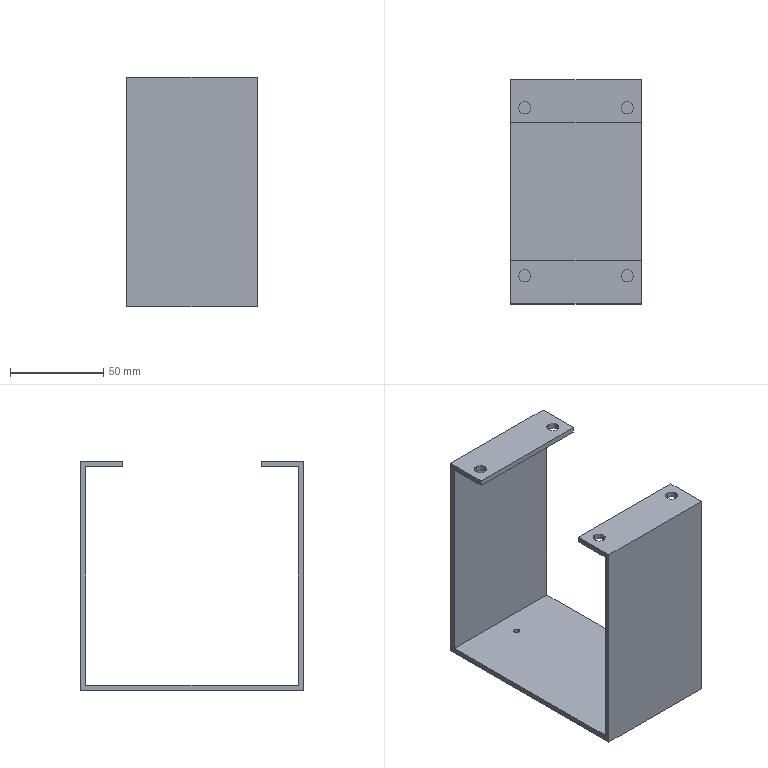Part | SolidWorks | features 3DProfileFeature 1, BaseBody 1, HoleWzd 1 | 1 solid | 26 faces | box 70 x 120 x 123 mm | volume 83550 mm3 | plane 14 | cylinder 12 | commonest cylinder face diameters 6.5 x8 3.3 x4
STEP:
#1=CARTESIAN_POINT('',(-36.65,15.,3.));
#2=VERTEX_POINT('',#1);
#3=CARTESIAN_POINT('',(-33.35,15.,3.));
#4=VERTEX_POINT('',#3);
#5=CARTESIAN_POINT('',(-35.,15.,3.));
#6=DIRECTION('',(0.,0.,1.));
#7=DIRECTION('',(1.,0.,0.));
#8=AXIS2_PLACEMENT_3D('',#5,#6,#7);
#9=CIRCLE('',#8,1.65);
#10=EDGE_CURVE('',#2,#4,#9,.T.);
#11=ORIENTED_EDGE('',*,*,#10,.T.);
#12=CARTESIAN_POINT('',(-33.35,15.,0.));
#13=VERTEX_POINT('',#12);
#14=CARTESIAN_POINT('',(-33.35,15.,0.));
#15=DIRECTION('',(0.,0.,-1.));
#16=VECTOR('',#15,1000.);
#17=LINE('',#14,#16);
#18=EDGE_CURVE('',#4,#13,#17,.T.);
#19=ORIENTED_EDGE('',*,*,#18,.T.);
#20=CARTESIAN_POINT('',(-36.65,15.,0.));
#21=VERTEX_POINT('',#20);
#22=CARTESIAN_POINT('',(-35.,15.,0.));
#23=DIRECTION('',(0.,0.,-1.));
#24=DIRECTION('',(-1.,0.,0.));
#25=AXIS2_PLACEMENT_3D('',#22,#23,#24);
#26=CIRCLE('',#25,1.65);
#27=EDGE_CURVE('',#13,#21,#26,.T.);
#28=ORIENTED_EDGE('',*,*,#27,.T.);
#29=CARTESIAN_POINT('',(-36.65,15.,0.));
#30=DIRECTION('',(0.,0.,-1.));
#31=VECTOR('',#30,1000.);
#32=LINE('',#29,#31);
#33=EDGE_CURVE('',#2,#21,#32,.T.);
#34=ORIENTED_EDGE('',*,*,#33,.F.);
#35=EDGE_LOOP('',(#11,#19,#28,#34));
#36=FACE_OUTER_BOUND('',#35,.T.);
#37=CARTESIAN_POINT('',(-35.,15.,0.));
#38=DIRECTION('',(0.,0.,-1.));
#39=DIRECTION('',(-1.,0.,0.));
#40=AXIS2_PLACEMENT_3D('',#37,#38,#39);
#41=CYLINDRICAL_SURFACE('',#40,1.65);
#42=ADVANCED_FACE('',(#36),#41,.F.);
#43=CARTESIAN_POINT('',(-36.65,105.,3.));
#44=VERTEX_POINT('',#43);
#45=CARTESIAN_POINT('',(-33.35,105.,3.));
#46=VERTEX_POINT('',#45);
#47=CARTESIAN_POINT('',(-35.,105.,3.));
#48=DIRECTION('',(0.,0.,1.));
#49=DIRECTION('',(1.,0.,0.));
#50=AXIS2_PLACEMENT_3D('',#47,#48,#49);
#51=CIRCLE('',#50,1.65);
#52=EDGE_CURVE('',#44,#46,#51,.T.);
#53=ORIENTED_EDGE('',*,*,#52,.T.);
#54=CARTESIAN_POINT('',(-33.35,105.,0.));
#55=VERTEX_POINT('',#54);
#56=CARTESIAN_POINT('',(-33.35,105.,0.));
#57=DIRECTION('',(0.,0.,-1.));
#58=VECTOR('',#57,1000.);
#59=LINE('',#56,#58);
#60=EDGE_CURVE('',#46,#55,#59,.T.);
#61=ORIENTED_EDGE('',*,*,#60,.T.);
#62=CARTESIAN_POINT('',(-36.65,105.,0.));
#63=VERTEX_POINT('',#62);
#64=CARTESIAN_POINT('',(-35.,105.,0.));
#65=DIRECTION('',(0.,0.,-1.));
#66=DIRECTION('',(-1.,0.,0.));
#67=AXIS2_PLACEMENT_3D('',#64,#65,#66);
#68=CIRCLE('',#67,1.65);
#69=EDGE_CURVE('',#55,#63,#68,.T.);
#70=ORIENTED_EDGE('',*,*,#69,.T.);
#71=CARTESIAN_POINT('',(-36.65,105.,0.));
#72=DIRECTION('',(0.,0.,-1.));
#73=VECTOR('',#72,1000.);
#74=LINE('',#71,#73);
#75=EDGE_CURVE('',#44,#63,#74,.T.);
#76=ORIENTED_EDGE('',*,*,#75,.F.);
#77=EDGE_LOOP('',(#53,#61,#70,#76));
#78=FACE_OUTER_BOUND('',#77,.T.);
#79=CARTESIAN_POINT('',(-35.,105.,0.));
#80=DIRECTION('',(0.,0.,-1.));
#81=DIRECTION('',(-1.,0.,0.));
#82=AXIS2_PLACEMENT_3D('',#79,#80,#81);
#83=CYLINDRICAL_SURFACE('',#82,1.65);
#84=ADVANCED_FACE('',(#78),#83,.F.);
#85=CARTESIAN_POINT('',(-7.5,101.75,120.));
#86=VERTEX_POINT('',#85);
#87=CARTESIAN_POINT('',(-7.5,108.25,120.));
#88=VERTEX_POINT('',#87);
#89=CARTESIAN_POINT('',(-7.5,105.,120.));
#90=DIRECTION('',(0.,0.,-1.));
#91=DIRECTION('',(0.,-1.,0.));
#92=AXIS2_PLACEMENT_3D('',#89,#90,#91);
#93=CIRCLE('',#92,3.25);
#94=EDGE_CURVE('',#86,#88,#93,.T.);
#95=ORIENTED_EDGE('',*,*,#94,.T.);
#96=CARTESIAN_POINT('',(-7.5,108.25,123.));
#97=VERTEX_POINT('',#96);
#98=CARTESIAN_POINT('',(-7.5,108.25,120.));
#99=DIRECTION('',(0.,0.,1.));
#100=VECTOR('',#99,1000.);
#101=LINE('',#98,#100);
#102=EDGE_CURVE('',#88,#97,#101,.T.);
#103=ORIENTED_EDGE('',*,*,#102,.T.);
#104=CARTESIAN_POINT('',(-7.5,101.75,123.));
#105=VERTEX_POINT('',#104);
#106=CARTESIAN_POINT('',(-7.5,105.,123.));
#107=DIRECTION('',(0.,0.,1.));
#108=DIRECTION('',(0.,-1.,0.));
#109=AXIS2_PLACEMENT_3D('',#106,#107,#108);
#110=CIRCLE('',#109,3.25);
#111=EDGE_CURVE('',#97,#105,#110,.T.);
#112=ORIENTED_EDGE('',*,*,#111,.T.);
#113=CARTESIAN_POINT('',(-7.5,101.75,120.));
#114=DIRECTION('',(0.,0.,1.));
#115=VECTOR('',#114,1000.);
#116=LINE('',#113,#115);
#117=EDGE_CURVE('',#86,#105,#116,.T.);
#118=ORIENTED_EDGE('',*,*,#117,.F.);
#119=EDGE_LOOP('',(#95,#103,#112,#118));
#120=FACE_OUTER_BOUND('',#119,.T.);
#121=CARTESIAN_POINT('',(-7.5,105.,120.));
#122=DIRECTION('',(0.,0.,1.));
#123=DIRECTION('',(0.,-1.,0.));
#124=AXIS2_PLACEMENT_3D('',#121,#122,#123);
#125=CYLINDRICAL_SURFACE('',#124,3.25);
#126=ADVANCED_FACE('',(#120),#125,.F.);
#127=CARTESIAN_POINT('',(-62.5,101.75,120.));
#128=VERTEX_POINT('',#127);
#129=CARTESIAN_POINT('',(-62.5,108.25,120.));
#130=VERTEX_POINT('',#129);
#131=CARTESIAN_POINT('',(-62.5,105.,120.));
#132=DIRECTION('',(0.,0.,-1.));
#133=DIRECTION('',(0.,-1.,0.));
#134=AXIS2_PLACEMENT_3D('',#131,#132,#133);
#135=CIRCLE('',#134,3.25);
#136=EDGE_CURVE('',#128,#130,#135,.T.);
#137=ORIENTED_EDGE('',*,*,#136,.T.);
#138=CARTESIAN_POINT('',(-62.5,108.25,123.));
#139=VERTEX_POINT('',#138);
#140=CARTESIAN_POINT('',(-62.5,108.25,120.));
#141=DIRECTION('',(0.,0.,1.));
#142=VECTOR('',#141,1000.);
#143=LINE('',#140,#142);
#144=EDGE_CURVE('',#130,#139,#143,.T.);
#145=ORIENTED_EDGE('',*,*,#144,.T.);
#146=CARTESIAN_POINT('',(-62.5,101.75,123.));
#147=VERTEX_POINT('',#146);
#148=CARTESIAN_POINT('',(-62.5,105.,123.));
#149=DIRECTION('',(0.,0.,-1.));
#150=DIRECTION('',(0.,-1.,0.));
#151=AXIS2_PLACEMENT_3D('',#148,#149,#150);
#152=CIRCLE('',#151,3.25);
#153=EDGE_CURVE('',#147,#139,#152,.T.);
#154=ORIENTED_EDGE('',*,*,#153,.F.);
#155=CARTESIAN_POINT('',(-62.5,101.75,120.));
#156=DIRECTION('',(0.,0.,1.));
#157=VECTOR('',#156,1000.);
#158=LINE('',#155,#157);
#159=EDGE_CURVE('',#128,#147,#158,.T.);
#160=ORIENTED_EDGE('',*,*,#159,.F.);
#161=EDGE_LOOP('',(#137,#145,#154,#160));
#162=FACE_OUTER_BOUND('',#161,.T.);
#163=CARTESIAN_POINT('',(-62.5,105.,120.));
#164=DIRECTION('',(0.,0.,1.));
#165=DIRECTION('',(0.,-1.,0.));
#166=AXIS2_PLACEMENT_3D('',#163,#164,#165);
#167=CYLINDRICAL_SURFACE('',#166,3.25);
#168=ADVANCED_FACE('',(#162),#167,.F.);
#169=CARTESIAN_POINT('',(-7.5,11.75,120.));
#170=VERTEX_POINT('',#169);
#171=CARTESIAN_POINT('',(-7.5,18.25,120.));
#172=VERTEX_POINT('',#171);
#173=CARTESIAN_POINT('',(-7.5,15.,120.));
#174=DIRECTION('',(0.,0.,-1.));
#175=DIRECTION('',(0.,-1.,0.));
#176=AXIS2_PLACEMENT_3D('',#173,#174,#175);
#177=CIRCLE('',#176,3.25);
#178=EDGE_CURVE('',#170,#172,#177,.T.);
#179=ORIENTED_EDGE('',*,*,#178,.T.);
#180=CARTESIAN_POINT('',(-7.5,18.25,123.));
#181=VERTEX_POINT('',#180);
#182=CARTESIAN_POINT('',(-7.5,18.25,120.));
#183=DIRECTION('',(0.,0.,1.));
#184=VECTOR('',#183,1000.);
#185=LINE('',#182,#184);
#186=EDGE_CURVE('',#172,#181,#185,.T.);
#187=ORIENTED_EDGE('',*,*,#186,.T.);
#188=CARTESIAN_POINT('',(-7.5,11.75,123.));
#189=VERTEX_POINT('',#188);
#190=CARTESIAN_POINT('',(-7.5,15.,123.));
#191=DIRECTION('',(0.,0.,-1.));
#192=DIRECTION('',(0.,-1.,0.));
#193=AXIS2_PLACEMENT_3D('',#190,#191,#192);
#194=CIRCLE('',#193,3.25);
#195=EDGE_CURVE('',#189,#181,#194,.T.);
#196=ORIENTED_EDGE('',*,*,#195,.F.);
#197=CARTESIAN_POINT('',(-7.5,11.75,120.));
#198=DIRECTION('',(0.,0.,1.));
#199=VECTOR('',#198,1000.);
#200=LINE('',#197,#199);
#201=EDGE_CURVE('',#170,#189,#200,.T.);
#202=ORIENTED_EDGE('',*,*,#201,.F.);
#203=EDGE_LOOP('',(#179,#187,#196,#202));
#204=FACE_OUTER_BOUND('',#203,.T.);
#205=CARTESIAN_POINT('',(-7.5,15.,120.));
#206=DIRECTION('',(0.,0.,1.));
#207=DIRECTION('',(0.,-1.,0.));
#208=AXIS2_PLACEMENT_3D('',#205,#206,#207);
#209=CYLINDRICAL_SURFACE('',#208,3.25);
#210=ADVANCED_FACE('',(#204),#209,.F.);
#211=CARTESIAN_POINT('',(-62.5,11.75,120.));
#212=VERTEX_POINT('',#211);
#213=CARTESIAN_POINT('',(-62.5,18.25,120.));
#214=VERTEX_POINT('',#213);
#215=CARTESIAN_POINT('',(-62.5,15.,120.));
#216=DIRECTION('',(0.,0.,-1.));
#217=DIRECTION('',(0.,-1.,0.));
#218=AXIS2_PLACEMENT_3D('',#215,#216,#217);
#219=CIRCLE('',#218,3.25);
#220=EDGE_CURVE('',#212,#214,#219,.T.);
#221=ORIENTED_EDGE('',*,*,#220,.T.);
#222=CARTESIAN_POINT('',(-62.5,18.25,123.));
#223=VERTEX_POINT('',#222);
#224=CARTESIAN_POINT('',(-62.5,18.25,120.));
#225=DIRECTION('',(0.,0.,1.));
#226=VECTOR('',#225,1000.);
#227=LINE('',#224,#226);
#228=EDGE_CURVE('',#214,#223,#227,.T.);
#229=ORIENTED_EDGE('',*,*,#228,.T.);
#230=CARTESIAN_POINT('',(-62.5,11.75,123.));
#231=VERTEX_POINT('',#230);
#232=CARTESIAN_POINT('',(-62.5,15.,123.));
#233=DIRECTION('',(0.,0.,-1.));
#234=DIRECTION('',(0.,-1.,0.));
#235=AXIS2_PLACEMENT_3D('',#232,#233,#234);
#236=CIRCLE('',#235,3.25);
#237=EDGE_CURVE('',#231,#223,#236,.T.);
#238=ORIENTED_EDGE('',*,*,#237,.F.);
#239=CARTESIAN_POINT('',(-62.5,11.75,120.));
#240=DIRECTION('',(0.,0.,1.));
#241=VECTOR('',#240,1000.);
#242=LINE('',#239,#241);
#243=EDGE_CURVE('',#212,#231,#242,.T.);
#244=ORIENTED_EDGE('',*,*,#243,.F.);
#245=EDGE_LOOP('',(#221,#229,#238,#244));
#246=FACE_OUTER_BOUND('',#245,.T.);
#247=CARTESIAN_POINT('',(-62.5,15.,120.));
#248=DIRECTION('',(0.,0.,1.));
#249=DIRECTION('',(0.,-1.,0.));
#250=AXIS2_PLACEMENT_3D('',#247,#248,#249);
#251=CYLINDRICAL_SURFACE('',#250,3.25);
#252=ADVANCED_FACE('',(#246),#251,.F.);
#253=ORIENTED_EDGE('',*,*,#102,.F.);
#254=CARTESIAN_POINT('',(-7.5,105.,120.));
#255=DIRECTION('',(0.,0.,-1.));
#256=DIRECTION('',(0.,-1.,0.));
#257=AXIS2_PLACEMENT_3D('',#254,#255,#256);
#258=CIRCLE('',#257,3.25);
#259=EDGE_CURVE('',#88,#86,#258,.T.);
#260=ORIENTED_EDGE('',*,*,#259,.T.);
#261=ORIENTED_EDGE('',*,*,#117,.T.);
#262=CARTESIAN_POINT('',(-7.5,105.,123.));
#263=DIRECTION('',(0.,0.,1.));
#264=DIRECTION('',(0.,-1.,0.));
#265=AXIS2_PLACEMENT_3D('',#262,#263,#264);
#266=CIRCLE('',#265,3.25);
#267=EDGE_CURVE('',#105,#97,#266,.T.);
#268=ORIENTED_EDGE('',*,*,#267,.T.);
#269=EDGE_LOOP('',(#253,#260,#261,#268));
#270=FACE_OUTER_BOUND('',#269,.T.);
#271=CARTESIAN_POINT('',(-7.5,105.,120.));
#272=DIRECTION('',(0.,0.,1.));
#273=DIRECTION('',(0.,-1.,0.));
#274=AXIS2_PLACEMENT_3D('',#271,#272,#273);
#275=CYLINDRICAL_SURFACE('',#274,3.25);
#276=ADVANCED_FACE('',(#270),#275,.F.);
#277=ORIENTED_EDGE('',*,*,#153,.T.);
#278=CARTESIAN_POINT('',(-62.5,105.,123.));
#279=DIRECTION('',(0.,0.,-1.));
#280=DIRECTION('',(0.,-1.,0.));
#281=AXIS2_PLACEMENT_3D('',#278,#279,#280);
#282=CIRCLE('',#281,3.25);
#283=EDGE_CURVE('',#139,#147,#282,.T.);
#284=ORIENTED_EDGE('',*,*,#283,.T.);
#285=EDGE_LOOP('',(#277,#284));
#286=FACE_BOUND('',#285,.T.);
#287=ORIENTED_EDGE('',*,*,#267,.F.);
#288=ORIENTED_EDGE('',*,*,#111,.F.);
#289=EDGE_LOOP('',(#287,#288));
#290=FACE_BOUND('',#289,.T.);
#291=CARTESIAN_POINT('',(0.,97.,123.));
#292=VERTEX_POINT('',#291);
#293=CARTESIAN_POINT('',(0.,120.,123.));
#294=VERTEX_POINT('',#293);
#295=CARTESIAN_POINT('',(0.,108.5,123.));
#296=DIRECTION('',(0.,1.,0.));
#297=VECTOR('',#296,1000.);
#298=LINE('',#295,#297);
#299=EDGE_CURVE('',#292,#294,#298,.T.);
#300=ORIENTED_EDGE('',*,*,#299,.T.);
#301=CARTESIAN_POINT('',(-70.,120.,123.));
#302=VERTEX_POINT('',#301);
#303=CARTESIAN_POINT('',(-35.,120.,123.));
#304=DIRECTION('',(-1.,0.,0.));
#305=VECTOR('',#304,1000.);
#306=LINE('',#303,#305);
#307=EDGE_CURVE('',#294,#302,#306,.T.);
#308=ORIENTED_EDGE('',*,*,#307,.T.);
#309=CARTESIAN_POINT('',(-70.,97.,123.));
#310=VERTEX_POINT('',#309);
#311=CARTESIAN_POINT('',(-70.,108.5,123.));
#312=DIRECTION('',(0.,-1.,0.));
#313=VECTOR('',#312,1000.);
#314=LINE('',#311,#313);
#315=EDGE_CURVE('',#302,#310,#314,.T.);
#316=ORIENTED_EDGE('',*,*,#315,.T.);
#317=CARTESIAN_POINT('',(-35.,97.,123.));
#318=DIRECTION('',(1.,0.,0.));
#319=VECTOR('',#318,1000.);
#320=LINE('',#317,#319);
#321=EDGE_CURVE('',#310,#292,#320,.T.);
#322=ORIENTED_EDGE('',*,*,#321,.T.);
#323=EDGE_LOOP('',(#300,#308,#316,#322));
#324=FACE_OUTER_BOUND('',#323,.T.);
#325=CARTESIAN_POINT('',(-70.,97.,123.));
#326=DIRECTION('',(0.,0.,1.));
#327=DIRECTION('',(1.,0.,0.));
#328=AXIS2_PLACEMENT_3D('',#325,#326,#327);
#329=PLANE('',#328);
#330=ADVANCED_FACE('',(#286,#290,#324),#329,.T.);
#331=ORIENTED_EDGE('',*,*,#136,.F.);
#332=CARTESIAN_POINT('',(-62.5,105.,120.));
#333=DIRECTION('',(0.,0.,-1.));
#334=DIRECTION('',(0.,-1.,0.));
#335=AXIS2_PLACEMENT_3D('',#332,#333,#334);
#336=CIRCLE('',#335,3.25);
#337=EDGE_CURVE('',#130,#128,#336,.T.);
#338=ORIENTED_EDGE('',*,*,#337,.F.);
#339=EDGE_LOOP('',(#331,#338));
#340=FACE_BOUND('',#339,.T.);
#341=ORIENTED_EDGE('',*,*,#94,.F.);
#342=ORIENTED_EDGE('',*,*,#259,.F.);
#343=EDGE_LOOP('',(#341,#342));
#344=FACE_BOUND('',#343,.T.);
#345=CARTESIAN_POINT('',(0.,117.,120.));
#346=VERTEX_POINT('',#345);
#347=CARTESIAN_POINT('',(-70.,117.,120.));
#348=VERTEX_POINT('',#347);
#349=CARTESIAN_POINT('',(-35.,117.,120.));
#350=DIRECTION('',(-1.,0.,0.));
#351=VECTOR('',#350,1000.);
#352=LINE('',#349,#351);
#353=EDGE_CURVE('',#346,#348,#352,.T.);
#354=ORIENTED_EDGE('',*,*,#353,.F.);
#355=CARTESIAN_POINT('',(0.,97.,120.));
#356=VERTEX_POINT('',#355);
#357=CARTESIAN_POINT('',(0.,107.,120.));
#358=DIRECTION('',(0.,1.,0.));
#359=VECTOR('',#358,1000.);
#360=LINE('',#357,#359);
#361=EDGE_CURVE('',#356,#346,#360,.T.);
#362=ORIENTED_EDGE('',*,*,#361,.F.);
#363=CARTESIAN_POINT('',(-70.,97.,120.));
#364=VERTEX_POINT('',#363);
#365=CARTESIAN_POINT('',(-35.,97.,120.));
#366=DIRECTION('',(1.,0.,0.));
#367=VECTOR('',#366,1000.);
#368=LINE('',#365,#367);
#369=EDGE_CURVE('',#364,#356,#368,.T.);
#370=ORIENTED_EDGE('',*,*,#369,.F.);
#371=CARTESIAN_POINT('',(-70.,107.,120.));
#372=DIRECTION('',(0.,-1.,0.));
#373=VECTOR('',#372,1000.);
#374=LINE('',#371,#373);
#375=EDGE_CURVE('',#348,#364,#374,.T.);
#376=ORIENTED_EDGE('',*,*,#375,.F.);
#377=EDGE_LOOP('',(#354,#362,#370,#376));
#378=FACE_OUTER_BOUND('',#377,.T.);
#379=CARTESIAN_POINT('',(-70.,97.,120.));
#380=DIRECTION('',(0.,0.,1.));
#381=DIRECTION('',(1.,0.,0.));
#382=AXIS2_PLACEMENT_3D('',#379,#380,#381);
#383=PLANE('',#382);
#384=ADVANCED_FACE('',(#340,#344,#378),#383,.F.);
#385=ORIENTED_EDGE('',*,*,#144,.F.);
#386=ORIENTED_EDGE('',*,*,#337,.T.);
#387=ORIENTED_EDGE('',*,*,#159,.T.);
#388=ORIENTED_EDGE('',*,*,#283,.F.);
#389=EDGE_LOOP('',(#385,#386,#387,#388));
#390=FACE_OUTER_BOUND('',#389,.T.);
#391=CARTESIAN_POINT('',(-62.5,105.,120.));
#392=DIRECTION('',(0.,0.,1.));
#393=DIRECTION('',(0.,-1.,0.));
#394=AXIS2_PLACEMENT_3D('',#391,#392,#393);
#395=CYLINDRICAL_SURFACE('',#394,3.25);
#396=ADVANCED_FACE('',(#390),#395,.F.);
#397=CARTESIAN_POINT('',(-70.,120.,0.));
#398=VERTEX_POINT('',#397);
#399=CARTESIAN_POINT('',(-70.,120.,61.5));
#400=DIRECTION('',(0.,0.,-1.));
#401=VECTOR('',#400,1000.);
#402=LINE('',#399,#401);
#403=EDGE_CURVE('',#302,#398,#402,.T.);
#404=ORIENTED_EDGE('',*,*,#403,.F.);
#405=ORIENTED_EDGE('',*,*,#307,.F.);
#406=CARTESIAN_POINT('',(0.,120.,0.));
#407=VERTEX_POINT('',#406);
#408=CARTESIAN_POINT('',(0.,120.,61.5));
#409=DIRECTION('',(0.,0.,1.));
#410=VECTOR('',#409,1000.);
#411=LINE('',#408,#410);
#412=EDGE_CURVE('',#407,#294,#411,.T.);
#413=ORIENTED_EDGE('',*,*,#412,.F.);
#414=CARTESIAN_POINT('',(-35.,120.,0.));
#415=DIRECTION('',(1.,0.,0.));
#416=VECTOR('',#415,1000.);
#417=LINE('',#414,#416);
#418=EDGE_CURVE('',#398,#407,#417,.T.);
#419=ORIENTED_EDGE('',*,*,#418,.F.);
#420=EDGE_LOOP('',(#404,#405,#413,#419));
#421=FACE_OUTER_BOUND('',#420,.T.);
#422=CARTESIAN_POINT('',(-70.,120.,0.));
#423=DIRECTION('',(0.,-1.,0.));
#424=DIRECTION('',(1.,0.,0.));
#425=AXIS2_PLACEMENT_3D('',#422,#423,#424);
#426=PLANE('',#425);
#427=ADVANCED_FACE('',(#421),#426,.F.);
#428=ORIENTED_EDGE('',*,*,#412,.T.);
#429=ORIENTED_EDGE('',*,*,#299,.F.);
#430=CARTESIAN_POINT('',(0.,97.,61.5));
#431=DIRECTION('',(0.,0.,1.));
#432=VECTOR('',#431,1000.);
#433=LINE('',#430,#432);
#434=EDGE_CURVE('',#356,#292,#433,.T.);
#435=ORIENTED_EDGE('',*,*,#434,.F.);
#436=ORIENTED_EDGE('',*,*,#361,.T.);
#437=CARTESIAN_POINT('',(0.,117.,3.));
#438=VERTEX_POINT('',#437);
#439=CARTESIAN_POINT('',(0.,117.,61.5));
#440=DIRECTION('',(0.,0.,1.));
#441=VECTOR('',#440,1000.);
#442=LINE('',#439,#441);
#443=EDGE_CURVE('',#438,#346,#442,.T.);
#444=ORIENTED_EDGE('',*,*,#443,.F.);
#445=CARTESIAN_POINT('',(0.,3.,3.));
#446=VERTEX_POINT('',#445);
#447=CARTESIAN_POINT('',(0.,60.,3.));
#448=DIRECTION('',(0.,1.,0.));
#449=VECTOR('',#448,1000.);
#450=LINE('',#447,#449);
#451=EDGE_CURVE('',#446,#438,#450,.T.);
#452=ORIENTED_EDGE('',*,*,#451,.F.);
#453=CARTESIAN_POINT('',(0.,3.,120.));
#454=VERTEX_POINT('',#453);
#455=CARTESIAN_POINT('',(0.,3.,61.5));
#456=DIRECTION('',(0.,0.,-1.));
#457=VECTOR('',#456,1000.);
#458=LINE('',#455,#457);
#459=EDGE_CURVE('',#454,#446,#458,.T.);
#460=ORIENTED_EDGE('',*,*,#459,.F.);
#461=CARTESIAN_POINT('',(0.,23.,120.));
#462=VERTEX_POINT('',#461);
#463=CARTESIAN_POINT('',(0.,60.,120.));
#464=DIRECTION('',(0.,-1.,0.));
#465=VECTOR('',#464,1000.);
#466=LINE('',#463,#465);
#467=EDGE_CURVE('',#462,#454,#466,.T.);
#468=ORIENTED_EDGE('',*,*,#467,.F.);
#469=CARTESIAN_POINT('',(0.,23.,123.));
#470=VERTEX_POINT('',#469);
#471=CARTESIAN_POINT('',(0.,23.,61.5));
#472=DIRECTION('',(0.,0.,-1.));
#473=VECTOR('',#472,1000.);
#474=LINE('',#471,#473);
#475=EDGE_CURVE('',#470,#462,#474,.T.);
#476=ORIENTED_EDGE('',*,*,#475,.F.);
#477=CARTESIAN_POINT('',(0.,0.,123.));
#478=VERTEX_POINT('',#477);
#479=CARTESIAN_POINT('',(0.,60.,123.));
#480=DIRECTION('',(0.,1.,0.));
#481=VECTOR('',#480,1000.);
#482=LINE('',#479,#481);
#483=EDGE_CURVE('',#478,#470,#482,.T.);
#484=ORIENTED_EDGE('',*,*,#483,.F.);
#485=CARTESIAN_POINT('',(0.,0.,0.));
#486=VERTEX_POINT('',#485);
#487=CARTESIAN_POINT('',(0.,0.,61.5));
#488=DIRECTION('',(0.,0.,1.));
#489=VECTOR('',#488,1000.);
#490=LINE('',#487,#489);
#491=EDGE_CURVE('',#486,#478,#490,.T.);
#492=ORIENTED_EDGE('',*,*,#491,.F.);
#493=CARTESIAN_POINT('',(0.,60.,0.));
#494=DIRECTION('',(0.,-1.,0.));
#495=VECTOR('',#494,1000.);
#496=LINE('',#493,#495);
#497=EDGE_CURVE('',#407,#486,#496,.T.);
#498=ORIENTED_EDGE('',*,*,#497,.F.);
#499=EDGE_LOOP('',(#428,#429,#435,#436,#444,#452,#460,#468,#476,#484,#492,#498));
#500=FACE_OUTER_BOUND('',#499,.T.);
#501=CARTESIAN_POINT('',(0.,0.,0.));
#502=DIRECTION('',(-1.,0.,0.));
#503=DIRECTION('',(0.,0.,1.));
#504=AXIS2_PLACEMENT_3D('',#501,#502,#503);
#505=PLANE('',#504);
#506=ADVANCED_FACE('',(#500),#505,.F.);
#507=ORIENTED_EDGE('',*,*,#369,.T.);
#508=ORIENTED_EDGE('',*,*,#434,.T.);
#509=ORIENTED_EDGE('',*,*,#321,.F.);
#510=CARTESIAN_POINT('',(-70.,97.,121.5));
#511=DIRECTION('',(0.,0.,-1.));
#512=VECTOR('',#511,1000.);
#513=LINE('',#510,#512);
#514=EDGE_CURVE('',#310,#364,#513,.T.);
#515=ORIENTED_EDGE('',*,*,#514,.T.);
#516=EDGE_LOOP('',(#507,#508,#509,#515));
#517=FACE_OUTER_BOUND('',#516,.T.);
#518=CARTESIAN_POINT('',(-70.,97.,123.));
#519=DIRECTION('',(0.,-1.,0.));
#520=DIRECTION('',(0.,0.,-1.));
#521=AXIS2_PLACEMENT_3D('',#518,#519,#520);
#522=PLANE('',#521);
#523=ADVANCED_FACE('',(#517),#522,.T.);
#524=CARTESIAN_POINT('',(-70.,0.,123.));
#525=VERTEX_POINT('',#524);
#526=CARTESIAN_POINT('',(-70.,0.,0.));
#527=VERTEX_POINT('',#526);
#528=CARTESIAN_POINT('',(-70.,0.,61.5));
#529=DIRECTION('',(0.,0.,-1.));
#530=VECTOR('',#529,1000.);
#531=LINE('',#528,#530);
#532=EDGE_CURVE('',#525,#527,#531,.T.);
#533=ORIENTED_EDGE('',*,*,#532,.F.);
#534=CARTESIAN_POINT('',(-70.,23.,123.));
#535=VERTEX_POINT('',#534);
#536=CARTESIAN_POINT('',(-70.,60.,123.));
#537=DIRECTION('',(0.,-1.,0.));
#538=VECTOR('',#537,1000.);
#539=LINE('',#536,#538);
#540=EDGE_CURVE('',#535,#525,#539,.T.);
#541=ORIENTED_EDGE('',*,*,#540,.F.);
#542=CARTESIAN_POINT('',(-70.,23.,120.));
#543=VERTEX_POINT('',#542);
#544=CARTESIAN_POINT('',(-70.,23.,61.5));
#545=DIRECTION('',(0.,0.,1.));
#546=VECTOR('',#545,1000.);
#547=LINE('',#544,#546);
#548=EDGE_CURVE('',#543,#535,#547,.T.);
#549=ORIENTED_EDGE('',*,*,#548,.F.);
#550=CARTESIAN_POINT('',(-70.,3.,120.));
#551=VERTEX_POINT('',#550);
#552=CARTESIAN_POINT('',(-70.,60.,120.));
#553=DIRECTION('',(0.,1.,0.));
#554=VECTOR('',#553,1000.);
#555=LINE('',#552,#554);
#556=EDGE_CURVE('',#551,#543,#555,.T.);
#557=ORIENTED_EDGE('',*,*,#556,.F.);
#558=CARTESIAN_POINT('',(-70.,3.,3.));
#559=VERTEX_POINT('',#558);
#560=CARTESIAN_POINT('',(-70.,3.,61.5));
#561=DIRECTION('',(0.,0.,1.));
#562=VECTOR('',#561,1000.);
#563=LINE('',#560,#562);
#564=EDGE_CURVE('',#559,#551,#563,.T.);
#565=ORIENTED_EDGE('',*,*,#564,.F.);
#566=CARTESIAN_POINT('',(-70.,117.,3.));
#567=VERTEX_POINT('',#566);
#568=CARTESIAN_POINT('',(-70.,60.,3.));
#569=DIRECTION('',(0.,-1.,0.));
#570=VECTOR('',#569,1000.);
#571=LINE('',#568,#570);
#572=EDGE_CURVE('',#567,#559,#571,.T.);
#573=ORIENTED_EDGE('',*,*,#572,.F.);
#574=CARTESIAN_POINT('',(-70.,117.,61.5));
#575=DIRECTION('',(0.,0.,-1.));
#576=VECTOR('',#575,1000.);
#577=LINE('',#574,#576);
#578=EDGE_CURVE('',#348,#567,#577,.T.);
#579=ORIENTED_EDGE('',*,*,#578,.F.);
#580=ORIENTED_EDGE('',*,*,#375,.T.);
#581=ORIENTED_EDGE('',*,*,#514,.F.);
#582=ORIENTED_EDGE('',*,*,#315,.F.);
#583=ORIENTED_EDGE('',*,*,#403,.T.);
#584=CARTESIAN_POINT('',(-70.,60.,0.));
#585=DIRECTION('',(0.,1.,0.));
#586=VECTOR('',#585,1000.);
#587=LINE('',#584,#586);
#588=EDGE_CURVE('',#527,#398,#587,.T.);
#589=ORIENTED_EDGE('',*,*,#588,.F.);
#590=EDGE_LOOP('',(#533,#541,#549,#557,#565,#573,#579,#580,#581,#582,#583,#589));
#591=FACE_OUTER_BOUND('',#590,.T.);
#592=CARTESIAN_POINT('',(-70.,0.,123.));
#593=DIRECTION('',(1.,0.,0.));
#594=DIRECTION('',(0.,0.,-1.));
#595=AXIS2_PLACEMENT_3D('',#592,#593,#594);
#596=PLANE('',#595);
#597=ADVANCED_FACE('',(#591),#596,.F.);
#598=ORIENTED_EDGE('',*,*,#578,.T.);
#599=CARTESIAN_POINT('',(-35.,117.,3.));
#600=DIRECTION('',(-1.,0.,0.));
#601=VECTOR('',#600,1000.);
#602=LINE('',#599,#601);
#603=EDGE_CURVE('',#438,#567,#602,.T.);
#604=ORIENTED_EDGE('',*,*,#603,.F.);
#605=ORIENTED_EDGE('',*,*,#443,.T.);
#606=ORIENTED_EDGE('',*,*,#353,.T.);
#607=EDGE_LOOP('',(#598,#604,#605,#606));
#608=FACE_OUTER_BOUND('',#607,.T.);
#609=CARTESIAN_POINT('',(-70.,117.,3.));
#610=DIRECTION('',(0.,1.,0.));
#611=DIRECTION('',(0.,0.,1.));
#612=AXIS2_PLACEMENT_3D('',#609,#610,#611);
#613=PLANE('',#612);
#614=ADVANCED_FACE('',(#608),#613,.F.);
#615=CARTESIAN_POINT('',(-35.,15.,0.));
#616=DIRECTION('',(0.,0.,-1.));
#617=DIRECTION('',(-1.,0.,0.));
#618=AXIS2_PLACEMENT_3D('',#615,#616,#617);
#619=CIRCLE('',#618,1.65);
#620=EDGE_CURVE('',#21,#13,#619,.T.);
#621=ORIENTED_EDGE('',*,*,#620,.F.);
#622=ORIENTED_EDGE('',*,*,#27,.F.);
#623=EDGE_LOOP('',(#621,#622));
#624=FACE_BOUND('',#623,.T.);
#625=CARTESIAN_POINT('',(-35.,105.,0.));
#626=DIRECTION('',(0.,0.,-1.));
#627=DIRECTION('',(-1.,0.,0.));
#628=AXIS2_PLACEMENT_3D('',#625,#626,#627);
#629=CIRCLE('',#628,1.65);
#630=EDGE_CURVE('',#63,#55,#629,.T.);
#631=ORIENTED_EDGE('',*,*,#630,.F.);
#632=ORIENTED_EDGE('',*,*,#69,.F.);
#633=EDGE_LOOP('',(#631,#632));
#634=FACE_BOUND('',#633,.T.);
#635=CARTESIAN_POINT('',(-35.,0.,0.));
#636=DIRECTION('',(1.,0.,0.));
#637=VECTOR('',#636,1000.);
#638=LINE('',#635,#637);
#639=EDGE_CURVE('',#527,#486,#638,.T.);
#640=ORIENTED_EDGE('',*,*,#639,.F.);
#641=ORIENTED_EDGE('',*,*,#588,.T.);
#642=ORIENTED_EDGE('',*,*,#418,.T.);
#643=ORIENTED_EDGE('',*,*,#497,.T.);
#644=EDGE_LOOP('',(#640,#641,#642,#643));
#645=FACE_OUTER_BOUND('',#644,.T.);
#646=CARTESIAN_POINT('',(-70.,0.,0.));
#647=DIRECTION('',(0.,0.,1.));
#648=DIRECTION('',(1.,0.,0.));
#649=AXIS2_PLACEMENT_3D('',#646,#647,#648);
#650=PLANE('',#649);
#651=ADVANCED_FACE('',(#624,#634,#645),#650,.F.);
#652=ORIENTED_EDGE('',*,*,#10,.F.);
#653=CARTESIAN_POINT('',(-35.,15.,3.));
#654=DIRECTION('',(0.,0.,1.));
#655=DIRECTION('',(1.,0.,0.));
#656=AXIS2_PLACEMENT_3D('',#653,#654,#655);
#657=CIRCLE('',#656,1.65);
#658=EDGE_CURVE('',#4,#2,#657,.T.);
#659=ORIENTED_EDGE('',*,*,#658,.F.);
#660=EDGE_LOOP('',(#652,#659));
#661=FACE_BOUND('',#660,.T.);
#662=ORIENTED_EDGE('',*,*,#52,.F.);
#663=CARTESIAN_POINT('',(-35.,105.,3.));
#664=DIRECTION('',(0.,0.,1.));
#665=DIRECTION('',(1.,0.,0.));
#666=AXIS2_PLACEMENT_3D('',#663,#664,#665);
#667=CIRCLE('',#666,1.65);
#668=EDGE_CURVE('',#46,#44,#667,.T.);
#669=ORIENTED_EDGE('',*,*,#668,.F.);
#670=EDGE_LOOP('',(#662,#669));
#671=FACE_BOUND('',#670,.T.);
#672=ORIENTED_EDGE('',*,*,#451,.T.);
#673=ORIENTED_EDGE('',*,*,#603,.T.);
#674=ORIENTED_EDGE('',*,*,#572,.T.);
#675=CARTESIAN_POINT('',(-35.,3.,3.));
#676=DIRECTION('',(1.,0.,0.));
#677=VECTOR('',#676,1000.);
#678=LINE('',#675,#677);
#679=EDGE_CURVE('',#559,#446,#678,.T.);
#680=ORIENTED_EDGE('',*,*,#679,.T.);
#681=EDGE_LOOP('',(#672,#673,#674,#680));
#682=FACE_OUTER_BOUND('',#681,.T.);
#683=CARTESIAN_POINT('',(-70.,3.,3.));
#684=DIRECTION('',(0.,0.,1.));
#685=DIRECTION('',(1.,0.,0.));
#686=AXIS2_PLACEMENT_3D('',#683,#684,#685);
#687=PLANE('',#686);
#688=ADVANCED_FACE('',(#661,#671,#682),#687,.T.);
#689=ORIENTED_EDGE('',*,*,#459,.T.);
#690=ORIENTED_EDGE('',*,*,#679,.F.);
#691=ORIENTED_EDGE('',*,*,#564,.T.);
#692=CARTESIAN_POINT('',(-35.,3.,120.));
#693=DIRECTION('',(-1.,0.,0.));
#694=VECTOR('',#693,1000.);
#695=LINE('',#692,#694);
#696=EDGE_CURVE('',#454,#551,#695,.T.);
#697=ORIENTED_EDGE('',*,*,#696,.F.);
#698=EDGE_LOOP('',(#689,#690,#691,#697));
#699=FACE_OUTER_BOUND('',#698,.T.);
#700=CARTESIAN_POINT('',(-70.,3.,120.));
#701=DIRECTION('',(0.,-1.,0.));
#702=DIRECTION('',(0.,0.,-1.));
#703=AXIS2_PLACEMENT_3D('',#700,#701,#702);
#704=PLANE('',#703);
#705=ADVANCED_FACE('',(#699),#704,.F.);
#706=ORIENTED_EDGE('',*,*,#178,.F.);
#707=CARTESIAN_POINT('',(-7.5,15.,120.));
#708=DIRECTION('',(0.,0.,-1.));
#709=DIRECTION('',(0.,-1.,0.));
#710=AXIS2_PLACEMENT_3D('',#707,#708,#709);
#711=CIRCLE('',#710,3.25);
#712=EDGE_CURVE('',#172,#170,#711,.T.);
#713=ORIENTED_EDGE('',*,*,#712,.F.);
#714=EDGE_LOOP('',(#706,#713));
#715=FACE_BOUND('',#714,.T.);
#716=ORIENTED_EDGE('',*,*,#220,.F.);
#717=CARTESIAN_POINT('',(-62.5,15.,120.));
#718=DIRECTION('',(0.,0.,-1.));
#719=DIRECTION('',(0.,-1.,0.));
#720=AXIS2_PLACEMENT_3D('',#717,#718,#719);
#721=CIRCLE('',#720,3.25);
#722=EDGE_CURVE('',#214,#212,#721,.T.);
#723=ORIENTED_EDGE('',*,*,#722,.F.);
#724=EDGE_LOOP('',(#716,#723));
#725=FACE_BOUND('',#724,.T.);
#726=ORIENTED_EDGE('',*,*,#556,.T.);
#727=CARTESIAN_POINT('',(-35.,23.,120.));
#728=DIRECTION('',(-1.,0.,0.));
#729=VECTOR('',#728,1000.);
#730=LINE('',#727,#729);
#731=EDGE_CURVE('',#462,#543,#730,.T.);
#732=ORIENTED_EDGE('',*,*,#731,.F.);
#733=ORIENTED_EDGE('',*,*,#467,.T.);
#734=ORIENTED_EDGE('',*,*,#696,.T.);
#735=EDGE_LOOP('',(#726,#732,#733,#734));
#736=FACE_OUTER_BOUND('',#735,.T.);
#737=CARTESIAN_POINT('',(-70.,3.,120.));
#738=DIRECTION('',(0.,0.,1.));
#739=DIRECTION('',(1.,0.,0.));
#740=AXIS2_PLACEMENT_3D('',#737,#738,#739);
#741=PLANE('',#740);
#742=ADVANCED_FACE('',(#715,#725,#736),#741,.F.);
#743=ORIENTED_EDGE('',*,*,#731,.T.);
#744=ORIENTED_EDGE('',*,*,#548,.T.);
#745=CARTESIAN_POINT('',(-35.,23.,123.));
#746=DIRECTION('',(1.,0.,0.));
#747=VECTOR('',#746,1000.);
#748=LINE('',#745,#747);
#749=EDGE_CURVE('',#535,#470,#748,.T.);
#750=ORIENTED_EDGE('',*,*,#749,.T.);
#751=ORIENTED_EDGE('',*,*,#475,.T.);
#752=EDGE_LOOP('',(#743,#744,#750,#751));
#753=FACE_OUTER_BOUND('',#752,.T.);
#754=CARTESIAN_POINT('',(0.,23.,120.));
#755=DIRECTION('',(0.,1.,0.));
#756=DIRECTION('',(-1.,0.,0.));
#757=AXIS2_PLACEMENT_3D('',#754,#755,#756);
#758=PLANE('',#757);
#759=ADVANCED_FACE('',(#753),#758,.T.);
#760=ORIENTED_EDGE('',*,*,#195,.T.);
#761=CARTESIAN_POINT('',(-7.5,15.,123.));
#762=DIRECTION('',(0.,0.,-1.));
#763=DIRECTION('',(0.,-1.,0.));
#764=AXIS2_PLACEMENT_3D('',#761,#762,#763);
#765=CIRCLE('',#764,3.25);
#766=EDGE_CURVE('',#181,#189,#765,.T.);
#767=ORIENTED_EDGE('',*,*,#766,.T.);
#768=EDGE_LOOP('',(#760,#767));
#769=FACE_BOUND('',#768,.T.);
#770=ORIENTED_EDGE('',*,*,#237,.T.);
#771=CARTESIAN_POINT('',(-62.5,15.,123.));
#772=DIRECTION('',(0.,0.,-1.));
#773=DIRECTION('',(0.,-1.,0.));
#774=AXIS2_PLACEMENT_3D('',#771,#772,#773);
#775=CIRCLE('',#774,3.25);
#776=EDGE_CURVE('',#223,#231,#775,.T.);
#777=ORIENTED_EDGE('',*,*,#776,.T.);
#778=EDGE_LOOP('',(#770,#777));
#779=FACE_BOUND('',#778,.T.);
#780=ORIENTED_EDGE('',*,*,#749,.F.);
#781=ORIENTED_EDGE('',*,*,#540,.T.);
#782=CARTESIAN_POINT('',(-35.,0.,123.));
#783=DIRECTION('',(1.,0.,0.));
#784=VECTOR('',#783,1000.);
#785=LINE('',#782,#784);
#786=EDGE_CURVE('',#525,#478,#785,.T.);
#787=ORIENTED_EDGE('',*,*,#786,.T.);
#788=ORIENTED_EDGE('',*,*,#483,.T.);
#789=EDGE_LOOP('',(#780,#781,#787,#788));
#790=FACE_OUTER_BOUND('',#789,.T.);
#791=CARTESIAN_POINT('',(-70.,0.,123.));
#792=DIRECTION('',(0.,0.,1.));
#793=DIRECTION('',(1.,0.,0.));
#794=AXIS2_PLACEMENT_3D('',#791,#792,#793);
#795=PLANE('',#794);
#796=ADVANCED_FACE('',(#769,#779,#790),#795,.T.);
#797=ORIENTED_EDGE('',*,*,#491,.T.);
#798=ORIENTED_EDGE('',*,*,#786,.F.);
#799=ORIENTED_EDGE('',*,*,#532,.T.);
#800=ORIENTED_EDGE('',*,*,#639,.T.);
#801=EDGE_LOOP('',(#797,#798,#799,#800));
#802=FACE_OUTER_BOUND('',#801,.T.);
#803=CARTESIAN_POINT('',(0.,0.,0.));
#804=DIRECTION('',(0.,1.,0.));
#805=DIRECTION('',(-1.,0.,0.));
#806=AXIS2_PLACEMENT_3D('',#803,#804,#805);
#807=PLANE('',#806);
#808=ADVANCED_FACE('',(#802),#807,.F.);
#809=ORIENTED_EDGE('',*,*,#186,.F.);
#810=ORIENTED_EDGE('',*,*,#712,.T.);
#811=ORIENTED_EDGE('',*,*,#201,.T.);
#812=ORIENTED_EDGE('',*,*,#766,.F.);
#813=EDGE_LOOP('',(#809,#810,#811,#812));
#814=FACE_OUTER_BOUND('',#813,.T.);
#815=CARTESIAN_POINT('',(-7.5,15.,120.));
#816=DIRECTION('',(0.,0.,1.));
#817=DIRECTION('',(0.,-1.,0.));
#818=AXIS2_PLACEMENT_3D('',#815,#816,#817);
#819=CYLINDRICAL_SURFACE('',#818,3.25);
#820=ADVANCED_FACE('',(#814),#819,.F.);
#821=ORIENTED_EDGE('',*,*,#228,.F.);
#822=ORIENTED_EDGE('',*,*,#722,.T.);
#823=ORIENTED_EDGE('',*,*,#243,.T.);
#824=ORIENTED_EDGE('',*,*,#776,.F.);
#825=EDGE_LOOP('',(#821,#822,#823,#824));
#826=FACE_OUTER_BOUND('',#825,.T.);
#827=CARTESIAN_POINT('',(-62.5,15.,120.));
#828=DIRECTION('',(0.,0.,1.));
#829=DIRECTION('',(0.,-1.,0.));
#830=AXIS2_PLACEMENT_3D('',#827,#828,#829);
#831=CYLINDRICAL_SURFACE('',#830,3.25);
#832=ADVANCED_FACE('',(#826),#831,.F.);
#833=ORIENTED_EDGE('',*,*,#60,.F.);
#834=ORIENTED_EDGE('',*,*,#668,.T.);
#835=ORIENTED_EDGE('',*,*,#75,.T.);
#836=ORIENTED_EDGE('',*,*,#630,.T.);
#837=EDGE_LOOP('',(#833,#834,#835,#836));
#838=FACE_OUTER_BOUND('',#837,.T.);
#839=CARTESIAN_POINT('',(-35.,105.,0.));
#840=DIRECTION('',(0.,0.,-1.));
#841=DIRECTION('',(-1.,0.,0.));
#842=AXIS2_PLACEMENT_3D('',#839,#840,#841);
#843=CYLINDRICAL_SURFACE('',#842,1.65);
#844=ADVANCED_FACE('',(#838),#843,.F.);
#845=ORIENTED_EDGE('',*,*,#18,.F.);
#846=ORIENTED_EDGE('',*,*,#658,.T.);
#847=ORIENTED_EDGE('',*,*,#33,.T.);
#848=ORIENTED_EDGE('',*,*,#620,.T.);
#849=EDGE_LOOP('',(#845,#846,#847,#848));
#850=FACE_OUTER_BOUND('',#849,.T.);
#851=CARTESIAN_POINT('',(-35.,15.,0.));
#852=DIRECTION('',(0.,0.,-1.));
#853=DIRECTION('',(-1.,0.,0.));
#854=AXIS2_PLACEMENT_3D('',#851,#852,#853);
#855=CYLINDRICAL_SURFACE('',#854,1.65);
#856=ADVANCED_FACE('',(#850),#855,.F.);
#857=CLOSED_SHELL('',(#42,#84,#126,#168,#210,#252,#276,#330,#384,#396,#427,#506,#523,#597,#614,#651,#688,#705,#742,#759,#796,#808,#820,#832,#844,#856));
#858=MANIFOLD_SOLID_BREP('',#857);
#859=CARTESIAN_POINT('',(0.,0.,0.));
#860=DIRECTION('',(0.,0.,1.));
#861=DIRECTION('',(1.,0.,0.));
#862=AXIS2_PLACEMENT_3D('',#859,#860,#861);
#863=(LENGTH_UNIT()NAMED_UNIT(*)SI_UNIT(.MILLI.,.METRE.));
#864=UNCERTAINTY_MEASURE_WITH_UNIT(LENGTH_MEASURE(0.00001),#863,'','');
#865=(NAMED_UNIT(*)PLANE_ANGLE_UNIT()SI_UNIT($,.RADIAN.));
#866=(NAMED_UNIT(*)SI_UNIT($,.STERADIAN.)SOLID_ANGLE_UNIT());
#867=(GEOMETRIC_REPRESENTATION_CONTEXT(3)GLOBAL_UNCERTAINTY_ASSIGNED_CONTEXT((#864))GLOBAL_UNIT_ASSIGNED_CONTEXT((#863,#865,#866))REPRESENTATION_CONTEXT('',''));
#868=ADVANCED_BREP_SHAPE_REPRESENTATION('',(#858,#862),#867);